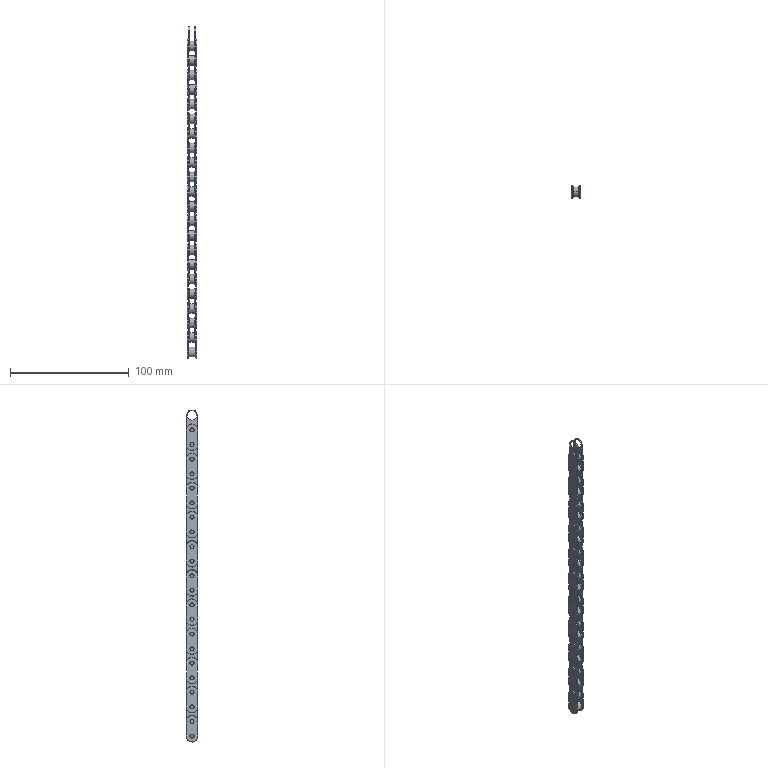Part | STEP file | 10 Chain Links v2 | 11 solids | 726 faces | box 8 x 10 x 280.1 mm | volume 12161 mm3 | cylinder 352 | plane 220 | torus 154 | commonest cylinder face diameters 3 x88 8 x88 9 x66 10 x66 0.4 x44